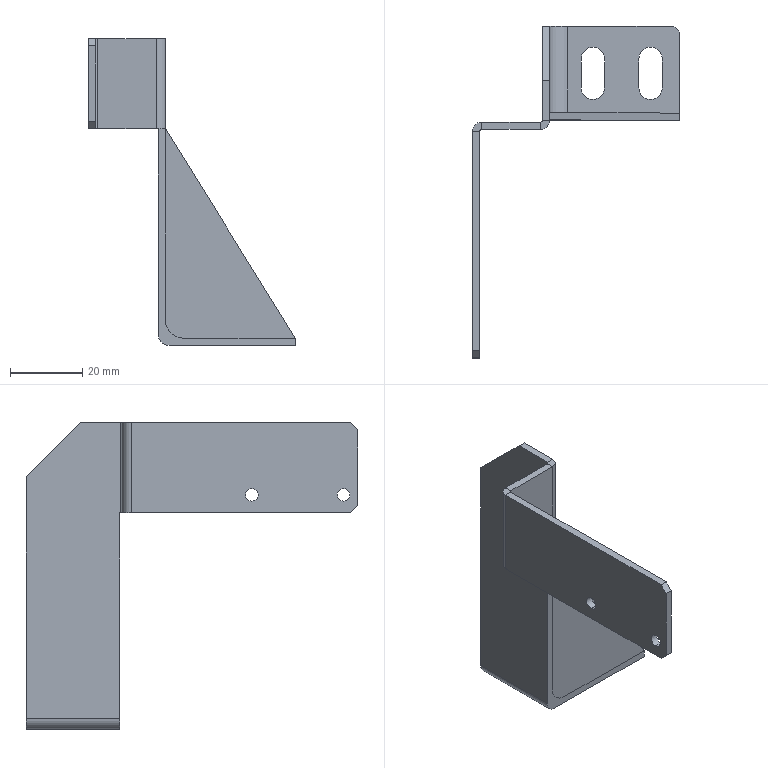Part | STEP file | Sensor Mount2_Default | 2 solids | 50 faces | box 57.322 x 91.966 x 85 mm | volume 12045 mm3 | plane 34 | cylinder 16 | commonest cylinder face diameters 3.5 x4 6.5 x4 1 x2 5 x2 10 x2 4 x1